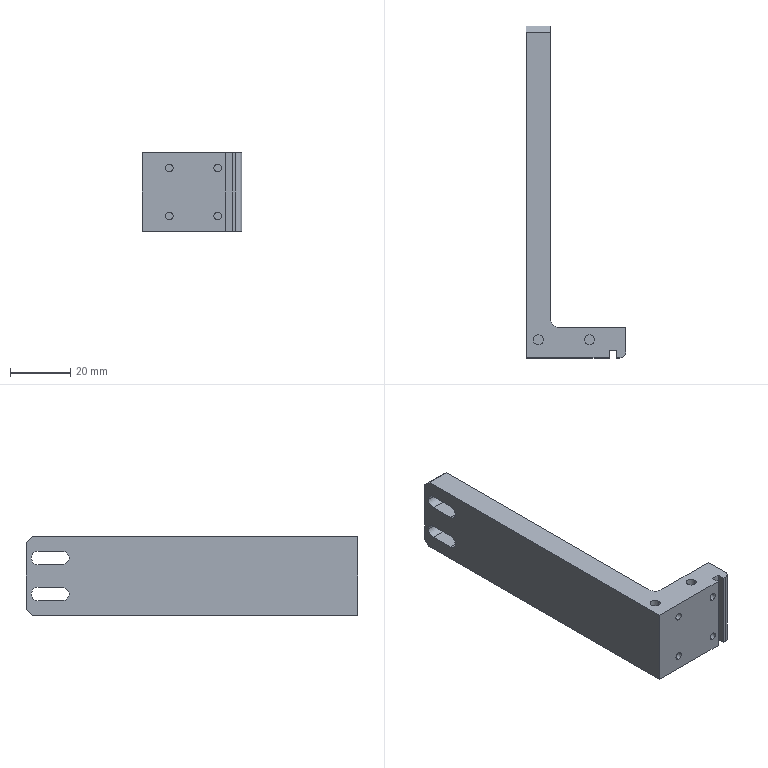Part | SolidWorks | features Fillet 2, HoleWzd 2, ICE 2, Chamfer 1, Extrusion 1, MirrorPattern 1 | 1 solid | 50 faces | box 33 x 110 x 26 mm | volume 27890 mm3 | plane 26 | cylinder 24 | commonest cylinder face diameters 2.5 x8 3.3 x8 4.5 x6 4 x1 6 x1
STEP:
#1=CARTESIAN_POINT('',(0.,108.25,-6.));
#2=VERTEX_POINT('',#1);
#3=CARTESIAN_POINT('',(0.,106.,-3.75));
#4=VERTEX_POINT('',#3);
#5=CARTESIAN_POINT('',(0.,106.,-6.));
#6=DIRECTION('',(1.,0.,0.));
#7=DIRECTION('',(0.,-1.,0.));
#8=AXIS2_PLACEMENT_3D('',#5,#6,#7);
#9=CIRCLE('',#8,2.25);
#10=EDGE_CURVE('',#2,#4,#9,.T.);
#11=ORIENTED_EDGE('',*,*,#10,.F.);
#12=CARTESIAN_POINT('',(8.,108.25,-6.));
#13=VERTEX_POINT('',#12);
#14=CARTESIAN_POINT('',(0.,108.25,-6.));
#15=DIRECTION('',(1.,0.,0.));
#16=VECTOR('',#15,1000.);
#17=LINE('',#14,#16);
#18=EDGE_CURVE('',#2,#13,#17,.T.);
#19=ORIENTED_EDGE('',*,*,#18,.T.);
#20=CARTESIAN_POINT('',(8.,106.,-3.75));
#21=VERTEX_POINT('',#20);
#22=CARTESIAN_POINT('',(8.,106.,-6.));
#23=DIRECTION('',(1.,0.,0.));
#24=DIRECTION('',(0.,-1.,0.));
#25=AXIS2_PLACEMENT_3D('',#22,#23,#24);
#26=CIRCLE('',#25,2.25);
#27=EDGE_CURVE('',#13,#21,#26,.T.);
#28=ORIENTED_EDGE('',*,*,#27,.T.);
#29=CARTESIAN_POINT('',(0.,106.,-3.75));
#30=DIRECTION('',(1.,0.,0.));
#31=VECTOR('',#30,1000.);
#32=LINE('',#29,#31);
#33=EDGE_CURVE('',#4,#21,#32,.T.);
#34=ORIENTED_EDGE('',*,*,#33,.F.);
#35=EDGE_LOOP('',(#11,#19,#28,#34));
#36=FACE_OUTER_BOUND('',#35,.T.);
#37=CARTESIAN_POINT('',(0.,106.,-6.));
#38=DIRECTION('',(1.,0.,0.));
#39=DIRECTION('',(0.,1.,0.));
#40=AXIS2_PLACEMENT_3D('',#37,#38,#39);
#41=CYLINDRICAL_SURFACE('',#40,2.25);
#42=ADVANCED_FACE('',(#36),#41,.F.);
#43=CARTESIAN_POINT('',(0.,108.25,6.));
#44=VERTEX_POINT('',#43);
#45=CARTESIAN_POINT('',(0.,106.,8.25));
#46=VERTEX_POINT('',#45);
#47=CARTESIAN_POINT('',(0.,106.,6.));
#48=DIRECTION('',(1.,0.,0.));
#49=DIRECTION('',(0.,1.,0.));
#50=AXIS2_PLACEMENT_3D('',#47,#48,#49);
#51=CIRCLE('',#50,2.25);
#52=EDGE_CURVE('',#44,#46,#51,.T.);
#53=ORIENTED_EDGE('',*,*,#52,.F.);
#54=CARTESIAN_POINT('',(8.,108.25,6.));
#55=VERTEX_POINT('',#54);
#56=CARTESIAN_POINT('',(0.,108.25,6.));
#57=DIRECTION('',(1.,0.,0.));
#58=VECTOR('',#57,1000.);
#59=LINE('',#56,#58);
#60=EDGE_CURVE('',#44,#55,#59,.T.);
#61=ORIENTED_EDGE('',*,*,#60,.T.);
#62=CARTESIAN_POINT('',(8.,106.,8.25));
#63=VERTEX_POINT('',#62);
#64=CARTESIAN_POINT('',(8.,106.,6.));
#65=DIRECTION('',(1.,0.,0.));
#66=DIRECTION('',(0.,1.,0.));
#67=AXIS2_PLACEMENT_3D('',#64,#65,#66);
#68=CIRCLE('',#67,2.25);
#69=EDGE_CURVE('',#55,#63,#68,.T.);
#70=ORIENTED_EDGE('',*,*,#69,.T.);
#71=CARTESIAN_POINT('',(0.,106.,8.25));
#72=DIRECTION('',(1.,0.,0.));
#73=VECTOR('',#72,1000.);
#74=LINE('',#71,#73);
#75=EDGE_CURVE('',#46,#63,#74,.T.);
#76=ORIENTED_EDGE('',*,*,#75,.F.);
#77=EDGE_LOOP('',(#53,#61,#70,#76));
#78=FACE_OUTER_BOUND('',#77,.T.);
#79=CARTESIAN_POINT('',(0.,106.,6.));
#80=DIRECTION('',(1.,0.,0.));
#81=DIRECTION('',(0.,1.,0.));
#82=AXIS2_PLACEMENT_3D('',#79,#80,#81);
#83=CYLINDRICAL_SURFACE('',#82,2.25);
#84=ADVANCED_FACE('',(#78),#83,.F.);
#85=CARTESIAN_POINT('',(25.,7.5,9.25));
#86=VERTEX_POINT('',#85);
#87=CARTESIAN_POINT('',(25.,7.5,6.75));
#88=VERTEX_POINT('',#87);
#89=CARTESIAN_POINT('',(25.,7.5,8.));
#90=DIRECTION('',(0.,-1.,0.));
#91=DIRECTION('',(0.,0.,-1.));
#92=AXIS2_PLACEMENT_3D('',#89,#90,#91);
#93=CIRCLE('',#92,1.25);
#94=EDGE_CURVE('',#86,#88,#93,.T.);
#95=ORIENTED_EDGE('',*,*,#94,.F.);
#96=CARTESIAN_POINT('',(25.,0.,9.25));
#97=VERTEX_POINT('',#96);
#98=CARTESIAN_POINT('',(25.,0.,9.25));
#99=DIRECTION('',(0.,-1.,0.));
#100=VECTOR('',#99,1000.);
#101=LINE('',#98,#100);
#102=EDGE_CURVE('',#86,#97,#101,.T.);
#103=ORIENTED_EDGE('',*,*,#102,.T.);
#104=CARTESIAN_POINT('',(25.,0.,6.75));
#105=VERTEX_POINT('',#104);
#106=CARTESIAN_POINT('',(25.,0.,8.));
#107=DIRECTION('',(0.,-1.,0.));
#108=DIRECTION('',(0.,0.,-1.));
#109=AXIS2_PLACEMENT_3D('',#106,#107,#108);
#110=CIRCLE('',#109,1.25);
#111=EDGE_CURVE('',#97,#105,#110,.T.);
#112=ORIENTED_EDGE('',*,*,#111,.T.);
#113=CARTESIAN_POINT('',(25.,0.,6.75));
#114=DIRECTION('',(0.,-1.,0.));
#115=VECTOR('',#114,1000.);
#116=LINE('',#113,#115);
#117=EDGE_CURVE('',#88,#105,#116,.T.);
#118=ORIENTED_EDGE('',*,*,#117,.F.);
#119=EDGE_LOOP('',(#95,#103,#112,#118));
#120=FACE_OUTER_BOUND('',#119,.T.);
#121=CARTESIAN_POINT('',(25.,0.,8.));
#122=DIRECTION('',(0.,-1.,0.));
#123=DIRECTION('',(0.,0.,-1.));
#124=AXIS2_PLACEMENT_3D('',#121,#122,#123);
#125=CYLINDRICAL_SURFACE('',#124,1.25);
#126=ADVANCED_FACE('',(#120),#125,.F.);
#127=CARTESIAN_POINT('',(9.,7.5,9.25));
#128=VERTEX_POINT('',#127);
#129=CARTESIAN_POINT('',(9.,7.5,6.75));
#130=VERTEX_POINT('',#129);
#131=CARTESIAN_POINT('',(9.,7.5,8.));
#132=DIRECTION('',(0.,-1.,0.));
#133=DIRECTION('',(0.,0.,-1.));
#134=AXIS2_PLACEMENT_3D('',#131,#132,#133);
#135=CIRCLE('',#134,1.25);
#136=EDGE_CURVE('',#128,#130,#135,.T.);
#137=ORIENTED_EDGE('',*,*,#136,.F.);
#138=CARTESIAN_POINT('',(9.,0.,9.25));
#139=VERTEX_POINT('',#138);
#140=CARTESIAN_POINT('',(9.,0.,9.25));
#141=DIRECTION('',(0.,-1.,0.));
#142=VECTOR('',#141,1000.);
#143=LINE('',#140,#142);
#144=EDGE_CURVE('',#128,#139,#143,.T.);
#145=ORIENTED_EDGE('',*,*,#144,.T.);
#146=CARTESIAN_POINT('',(9.,0.,6.75));
#147=VERTEX_POINT('',#146);
#148=CARTESIAN_POINT('',(9.,0.,8.));
#149=DIRECTION('',(0.,-1.,0.));
#150=DIRECTION('',(0.,0.,-1.));
#151=AXIS2_PLACEMENT_3D('',#148,#149,#150);
#152=CIRCLE('',#151,1.25);
#153=EDGE_CURVE('',#139,#147,#152,.T.);
#154=ORIENTED_EDGE('',*,*,#153,.T.);
#155=CARTESIAN_POINT('',(9.,0.,6.75));
#156=DIRECTION('',(0.,-1.,0.));
#157=VECTOR('',#156,1000.);
#158=LINE('',#155,#157);
#159=EDGE_CURVE('',#130,#147,#158,.T.);
#160=ORIENTED_EDGE('',*,*,#159,.F.);
#161=EDGE_LOOP('',(#137,#145,#154,#160));
#162=FACE_OUTER_BOUND('',#161,.T.);
#163=CARTESIAN_POINT('',(9.,0.,8.));
#164=DIRECTION('',(0.,-1.,0.));
#165=DIRECTION('',(0.,0.,-1.));
#166=AXIS2_PLACEMENT_3D('',#163,#164,#165);
#167=CYLINDRICAL_SURFACE('',#166,1.25);
#168=ADVANCED_FACE('',(#162),#167,.F.);
#169=CARTESIAN_POINT('',(9.,7.5,-6.75));
#170=VERTEX_POINT('',#169);
#171=CARTESIAN_POINT('',(9.,7.5,-9.25));
#172=VERTEX_POINT('',#171);
#173=CARTESIAN_POINT('',(9.,7.5,-8.));
#174=DIRECTION('',(0.,-1.,0.));
#175=DIRECTION('',(0.,0.,-1.));
#176=AXIS2_PLACEMENT_3D('',#173,#174,#175);
#177=CIRCLE('',#176,1.25);
#178=EDGE_CURVE('',#170,#172,#177,.T.);
#179=ORIENTED_EDGE('',*,*,#178,.F.);
#180=CARTESIAN_POINT('',(9.,0.,-6.75));
#181=VERTEX_POINT('',#180);
#182=CARTESIAN_POINT('',(9.,0.,-6.75));
#183=DIRECTION('',(0.,-1.,0.));
#184=VECTOR('',#183,1000.);
#185=LINE('',#182,#184);
#186=EDGE_CURVE('',#170,#181,#185,.T.);
#187=ORIENTED_EDGE('',*,*,#186,.T.);
#188=CARTESIAN_POINT('',(9.,0.,-9.25));
#189=VERTEX_POINT('',#188);
#190=CARTESIAN_POINT('',(9.,0.,-8.));
#191=DIRECTION('',(0.,-1.,0.));
#192=DIRECTION('',(0.,0.,-1.));
#193=AXIS2_PLACEMENT_3D('',#190,#191,#192);
#194=CIRCLE('',#193,1.25);
#195=EDGE_CURVE('',#181,#189,#194,.T.);
#196=ORIENTED_EDGE('',*,*,#195,.T.);
#197=CARTESIAN_POINT('',(9.,0.,-9.25));
#198=DIRECTION('',(0.,-1.,0.));
#199=VECTOR('',#198,1000.);
#200=LINE('',#197,#199);
#201=EDGE_CURVE('',#172,#189,#200,.T.);
#202=ORIENTED_EDGE('',*,*,#201,.F.);
#203=EDGE_LOOP('',(#179,#187,#196,#202));
#204=FACE_OUTER_BOUND('',#203,.T.);
#205=CARTESIAN_POINT('',(9.,0.,-8.));
#206=DIRECTION('',(0.,-1.,0.));
#207=DIRECTION('',(0.,0.,-1.));
#208=AXIS2_PLACEMENT_3D('',#205,#206,#207);
#209=CYLINDRICAL_SURFACE('',#208,1.25);
#210=ADVANCED_FACE('',(#204),#209,.F.);
#211=CARTESIAN_POINT('',(25.,7.5,-6.75));
#212=VERTEX_POINT('',#211);
#213=CARTESIAN_POINT('',(25.,7.5,-9.25));
#214=VERTEX_POINT('',#213);
#215=CARTESIAN_POINT('',(25.,7.5,-8.));
#216=DIRECTION('',(0.,-1.,0.));
#217=DIRECTION('',(0.,0.,-1.));
#218=AXIS2_PLACEMENT_3D('',#215,#216,#217);
#219=CIRCLE('',#218,1.25);
#220=EDGE_CURVE('',#212,#214,#219,.T.);
#221=ORIENTED_EDGE('',*,*,#220,.F.);
#222=CARTESIAN_POINT('',(25.,0.,-6.75));
#223=VERTEX_POINT('',#222);
#224=CARTESIAN_POINT('',(25.,0.,-6.75));
#225=DIRECTION('',(0.,-1.,0.));
#226=VECTOR('',#225,1000.);
#227=LINE('',#224,#226);
#228=EDGE_CURVE('',#212,#223,#227,.T.);
#229=ORIENTED_EDGE('',*,*,#228,.T.);
#230=CARTESIAN_POINT('',(25.,0.,-9.25));
#231=VERTEX_POINT('',#230);
#232=CARTESIAN_POINT('',(25.,0.,-8.));
#233=DIRECTION('',(0.,-1.,0.));
#234=DIRECTION('',(0.,0.,-1.));
#235=AXIS2_PLACEMENT_3D('',#232,#233,#234);
#236=CIRCLE('',#235,1.25);
#237=EDGE_CURVE('',#223,#231,#236,.T.);
#238=ORIENTED_EDGE('',*,*,#237,.T.);
#239=CARTESIAN_POINT('',(25.,0.,-9.25));
#240=DIRECTION('',(0.,-1.,0.));
#241=VECTOR('',#240,1000.);
#242=LINE('',#239,#241);
#243=EDGE_CURVE('',#214,#231,#242,.T.);
#244=ORIENTED_EDGE('',*,*,#243,.F.);
#245=EDGE_LOOP('',(#221,#229,#238,#244));
#246=FACE_OUTER_BOUND('',#245,.T.);
#247=CARTESIAN_POINT('',(25.,0.,-8.));
#248=DIRECTION('',(0.,-1.,0.));
#249=DIRECTION('',(0.,0.,-1.));
#250=AXIS2_PLACEMENT_3D('',#247,#248,#249);
#251=CYLINDRICAL_SURFACE('',#250,1.25);
#252=ADVANCED_FACE('',(#246),#251,.F.);
#253=CARTESIAN_POINT('',(22.65,6.,-2.9));
#254=VERTEX_POINT('',#253);
#255=CARTESIAN_POINT('',(19.35,6.,-2.9));
#256=VERTEX_POINT('',#255);
#257=CARTESIAN_POINT('',(21.,6.,-2.9));
#258=DIRECTION('',(0.,0.,-1.));
#259=DIRECTION('',(-1.,0.,0.));
#260=AXIS2_PLACEMENT_3D('',#257,#258,#259);
#261=CIRCLE('',#260,1.65);
#262=EDGE_CURVE('',#254,#256,#261,.T.);
#263=ORIENTED_EDGE('',*,*,#262,.F.);
#264=CARTESIAN_POINT('',(22.65,6.,-13.));
#265=VERTEX_POINT('',#264);
#266=CARTESIAN_POINT('',(22.65,6.,-13.));
#267=DIRECTION('',(0.,0.,-1.));
#268=VECTOR('',#267,1000.);
#269=LINE('',#266,#268);
#270=EDGE_CURVE('',#254,#265,#269,.T.);
#271=ORIENTED_EDGE('',*,*,#270,.T.);
#272=CARTESIAN_POINT('',(19.35,6.,-13.));
#273=VERTEX_POINT('',#272);
#274=CARTESIAN_POINT('',(21.,6.,-13.));
#275=DIRECTION('',(0.,0.,-1.));
#276=DIRECTION('',(-1.,0.,0.));
#277=AXIS2_PLACEMENT_3D('',#274,#275,#276);
#278=CIRCLE('',#277,1.65);
#279=EDGE_CURVE('',#265,#273,#278,.T.);
#280=ORIENTED_EDGE('',*,*,#279,.T.);
#281=CARTESIAN_POINT('',(19.35,6.,-13.));
#282=DIRECTION('',(0.,0.,-1.));
#283=VECTOR('',#282,1000.);
#284=LINE('',#281,#283);
#285=EDGE_CURVE('',#256,#273,#284,.T.);
#286=ORIENTED_EDGE('',*,*,#285,.F.);
#287=EDGE_LOOP('',(#263,#271,#280,#286));
#288=FACE_OUTER_BOUND('',#287,.T.);
#289=CARTESIAN_POINT('',(21.,6.,-13.));
#290=DIRECTION('',(0.,0.,-1.));
#291=DIRECTION('',(-1.,0.,0.));
#292=AXIS2_PLACEMENT_3D('',#289,#290,#291);
#293=CYLINDRICAL_SURFACE('',#292,1.65);
#294=ADVANCED_FACE('',(#288),#293,.F.);
#295=CARTESIAN_POINT('',(5.65,6.,-2.9));
#296=VERTEX_POINT('',#295);
#297=CARTESIAN_POINT('',(2.35,6.,-2.9));
#298=VERTEX_POINT('',#297);
#299=CARTESIAN_POINT('',(4.,6.,-2.9));
#300=DIRECTION('',(0.,0.,-1.));
#301=DIRECTION('',(-1.,0.,0.));
#302=AXIS2_PLACEMENT_3D('',#299,#300,#301);
#303=CIRCLE('',#302,1.65);
#304=EDGE_CURVE('',#296,#298,#303,.T.);
#305=ORIENTED_EDGE('',*,*,#304,.F.);
#306=CARTESIAN_POINT('',(5.65,6.,-13.));
#307=VERTEX_POINT('',#306);
#308=CARTESIAN_POINT('',(5.65,6.,-13.));
#309=DIRECTION('',(0.,0.,-1.));
#310=VECTOR('',#309,1000.);
#311=LINE('',#308,#310);
#312=EDGE_CURVE('',#296,#307,#311,.T.);
#313=ORIENTED_EDGE('',*,*,#312,.T.);
#314=CARTESIAN_POINT('',(2.35,6.,-13.));
#315=VERTEX_POINT('',#314);
#316=CARTESIAN_POINT('',(4.,6.,-13.));
#317=DIRECTION('',(0.,0.,-1.));
#318=DIRECTION('',(-1.,0.,0.));
#319=AXIS2_PLACEMENT_3D('',#316,#317,#318);
#320=CIRCLE('',#319,1.65);
#321=EDGE_CURVE('',#307,#315,#320,.T.);
#322=ORIENTED_EDGE('',*,*,#321,.T.);
#323=CARTESIAN_POINT('',(2.35,6.,-13.));
#324=DIRECTION('',(0.,0.,-1.));
#325=VECTOR('',#324,1000.);
#326=LINE('',#323,#325);
#327=EDGE_CURVE('',#298,#315,#326,.T.);
#328=ORIENTED_EDGE('',*,*,#327,.F.);
#329=EDGE_LOOP('',(#305,#313,#322,#328));
#330=FACE_OUTER_BOUND('',#329,.T.);
#331=CARTESIAN_POINT('',(4.,6.,-13.));
#332=DIRECTION('',(0.,0.,-1.));
#333=DIRECTION('',(-1.,0.,0.));
#334=AXIS2_PLACEMENT_3D('',#331,#332,#333);
#335=CYLINDRICAL_SURFACE('',#334,1.65);
#336=ADVANCED_FACE('',(#330),#335,.F.);
#337=CARTESIAN_POINT('',(19.35,6.,2.9));
#338=VERTEX_POINT('',#337);
#339=CARTESIAN_POINT('',(22.65,6.,2.9));
#340=VERTEX_POINT('',#339);
#341=CARTESIAN_POINT('',(21.,6.,2.9));
#342=DIRECTION('',(0.,0.,1.));
#343=DIRECTION('',(1.,0.,0.));
#344=AXIS2_PLACEMENT_3D('',#341,#342,#343);
#345=CIRCLE('',#344,1.65);
#346=EDGE_CURVE('',#338,#340,#345,.T.);
#347=ORIENTED_EDGE('',*,*,#346,.F.);
#348=CARTESIAN_POINT('',(19.35,6.,13.));
#349=VERTEX_POINT('',#348);
#350=CARTESIAN_POINT('',(19.35,6.,13.));
#351=DIRECTION('',(0.,0.,1.));
#352=VECTOR('',#351,1000.);
#353=LINE('',#350,#352);
#354=EDGE_CURVE('',#338,#349,#353,.T.);
#355=ORIENTED_EDGE('',*,*,#354,.T.);
#356=CARTESIAN_POINT('',(22.65,6.,13.));
#357=VERTEX_POINT('',#356);
#358=CARTESIAN_POINT('',(21.,6.,13.));
#359=DIRECTION('',(0.,0.,1.));
#360=DIRECTION('',(1.,0.,0.));
#361=AXIS2_PLACEMENT_3D('',#358,#359,#360);
#362=CIRCLE('',#361,1.65);
#363=EDGE_CURVE('',#349,#357,#362,.T.);
#364=ORIENTED_EDGE('',*,*,#363,.T.);
#365=CARTESIAN_POINT('',(22.65,6.,13.));
#366=DIRECTION('',(0.,0.,1.));
#367=VECTOR('',#366,1000.);
#368=LINE('',#365,#367);
#369=EDGE_CURVE('',#340,#357,#368,.T.);
#370=ORIENTED_EDGE('',*,*,#369,.F.);
#371=EDGE_LOOP('',(#347,#355,#364,#370));
#372=FACE_OUTER_BOUND('',#371,.T.);
#373=CARTESIAN_POINT('',(21.,6.,13.));
#374=DIRECTION('',(0.,0.,1.));
#375=DIRECTION('',(1.,0.,0.));
#376=AXIS2_PLACEMENT_3D('',#373,#374,#375);
#377=CYLINDRICAL_SURFACE('',#376,1.65);
#378=ADVANCED_FACE('',(#372),#377,.F.);
#379=CARTESIAN_POINT('',(2.35,6.,2.9));
#380=VERTEX_POINT('',#379);
#381=CARTESIAN_POINT('',(5.65,6.,2.9));
#382=VERTEX_POINT('',#381);
#383=CARTESIAN_POINT('',(4.,6.,2.9));
#384=DIRECTION('',(0.,0.,1.));
#385=DIRECTION('',(1.,0.,0.));
#386=AXIS2_PLACEMENT_3D('',#383,#384,#385);
#387=CIRCLE('',#386,1.65);
#388=EDGE_CURVE('',#380,#382,#387,.T.);
#389=ORIENTED_EDGE('',*,*,#388,.F.);
#390=CARTESIAN_POINT('',(2.35,6.,13.));
#391=VERTEX_POINT('',#390);
#392=CARTESIAN_POINT('',(2.35,6.,13.));
#393=DIRECTION('',(0.,0.,1.));
#394=VECTOR('',#393,1000.);
#395=LINE('',#392,#394);
#396=EDGE_CURVE('',#380,#391,#395,.T.);
#397=ORIENTED_EDGE('',*,*,#396,.T.);
#398=CARTESIAN_POINT('',(5.65,6.,13.));
#399=VERTEX_POINT('',#398);
#400=CARTESIAN_POINT('',(4.,6.,13.));
#401=DIRECTION('',(0.,0.,1.));
#402=DIRECTION('',(1.,0.,0.));
#403=AXIS2_PLACEMENT_3D('',#400,#401,#402);
#404=CIRCLE('',#403,1.65);
#405=EDGE_CURVE('',#391,#399,#404,.T.);
#406=ORIENTED_EDGE('',*,*,#405,.T.);
#407=CARTESIAN_POINT('',(5.65,6.,13.));
#408=DIRECTION('',(0.,0.,1.));
#409=VECTOR('',#408,1000.);
#410=LINE('',#407,#409);
#411=EDGE_CURVE('',#382,#399,#410,.T.);
#412=ORIENTED_EDGE('',*,*,#411,.F.);
#413=EDGE_LOOP('',(#389,#397,#406,#412));
#414=FACE_OUTER_BOUND('',#413,.T.);
#415=CARTESIAN_POINT('',(4.,6.,13.));
#416=DIRECTION('',(0.,0.,1.));
#417=DIRECTION('',(1.,0.,0.));
#418=AXIS2_PLACEMENT_3D('',#415,#416,#417);
#419=CYLINDRICAL_SURFACE('',#418,1.65);
#420=ADVANCED_FACE('',(#414),#419,.F.);
#421=CARTESIAN_POINT('',(30.,0.,-13.));
#422=VERTEX_POINT('',#421);
#423=CARTESIAN_POINT('',(31.,0.,-13.));
#424=VERTEX_POINT('',#423);
#425=CARTESIAN_POINT('',(0.,0.,-13.));
#426=DIRECTION('',(1.,0.,0.));
#427=VECTOR('',#426,1000.);
#428=LINE('',#425,#427);
#429=EDGE_CURVE('',#422,#424,#428,.T.);
#430=ORIENTED_EDGE('',*,*,#429,.T.);
#431=CARTESIAN_POINT('',(31.,0.,13.));
#432=VERTEX_POINT('',#431);
#433=CARTESIAN_POINT('',(31.,0.,13.));
#434=DIRECTION('',(0.,0.,1.));
#435=VECTOR('',#434,1000.);
#436=LINE('',#433,#435);
#437=EDGE_CURVE('',#424,#432,#436,.T.);
#438=ORIENTED_EDGE('',*,*,#437,.T.);
#439=CARTESIAN_POINT('',(30.,0.,13.));
#440=VERTEX_POINT('',#439);
#441=CARTESIAN_POINT('',(0.,0.,13.));
#442=DIRECTION('',(1.,0.,0.));
#443=VECTOR('',#442,1000.);
#444=LINE('',#441,#443);
#445=EDGE_CURVE('',#440,#432,#444,.T.);
#446=ORIENTED_EDGE('',*,*,#445,.F.);
#447=CARTESIAN_POINT('',(30.,0.,-13.));
#448=DIRECTION('',(0.,0.,1.));
#449=VECTOR('',#448,1000.);
#450=LINE('',#447,#449);
#451=EDGE_CURVE('',#422,#440,#450,.T.);
#452=ORIENTED_EDGE('',*,*,#451,.F.);
#453=EDGE_LOOP('',(#430,#438,#446,#452));
#454=FACE_OUTER_BOUND('',#453,.T.);
#455=CARTESIAN_POINT('',(0.,0.,13.));
#456=DIRECTION('',(0.,1.,0.));
#457=DIRECTION('',(0.,0.,1.));
#458=AXIS2_PLACEMENT_3D('',#455,#456,#457);
#459=PLANE('',#458);
#460=ADVANCED_FACE('',(#454),#459,.F.);
#461=CARTESIAN_POINT('',(0.,98.,-8.25));
#462=VERTEX_POINT('',#461);
#463=CARTESIAN_POINT('',(0.,106.,-8.25));
#464=VERTEX_POINT('',#463);
#465=CARTESIAN_POINT('',(0.,106.,-8.25));
#466=DIRECTION('',(0.,1.,0.));
#467=VECTOR('',#466,1000.);
#468=LINE('',#465,#467);
#469=EDGE_CURVE('',#462,#464,#468,.T.);
#470=ORIENTED_EDGE('',*,*,#469,.T.);
#471=CARTESIAN_POINT('',(0.,106.,-6.));
#472=DIRECTION('',(1.,0.,0.));
#473=DIRECTION('',(0.,-1.,0.));
#474=AXIS2_PLACEMENT_3D('',#471,#472,#473);
#475=CIRCLE('',#474,2.25);
#476=EDGE_CURVE('',#464,#2,#475,.T.);
#477=ORIENTED_EDGE('',*,*,#476,.T.);
#478=ORIENTED_EDGE('',*,*,#10,.T.);
#479=CARTESIAN_POINT('',(0.,98.,-3.75));
#480=VERTEX_POINT('',#479);
#481=CARTESIAN_POINT('',(0.,106.,-3.75));
#482=DIRECTION('',(0.,-1.,0.));
#483=VECTOR('',#482,1000.);
#484=LINE('',#481,#483);
#485=EDGE_CURVE('',#4,#480,#484,.T.);
#486=ORIENTED_EDGE('',*,*,#485,.T.);
#487=CARTESIAN_POINT('',(0.,98.,-6.));
#488=DIRECTION('',(1.,0.,0.));
#489=DIRECTION('',(0.,-1.,0.));
#490=AXIS2_PLACEMENT_3D('',#487,#488,#489);
#491=CIRCLE('',#490,2.25);
#492=EDGE_CURVE('',#480,#462,#491,.T.);
#493=ORIENTED_EDGE('',*,*,#492,.T.);
#494=EDGE_LOOP('',(#470,#477,#478,#486,#493));
#495=FACE_BOUND('',#494,.T.);
#496=CARTESIAN_POINT('',(0.,98.,3.75));
#497=VERTEX_POINT('',#496);
#498=CARTESIAN_POINT('',(0.,106.,3.75));
#499=VERTEX_POINT('',#498);
#500=CARTESIAN_POINT('',(0.,106.,3.75));
#501=DIRECTION('',(0.,1.,0.));
#502=VECTOR('',#501,1000.);
#503=LINE('',#500,#502);
#504=EDGE_CURVE('',#497,#499,#503,.T.);
#505=ORIENTED_EDGE('',*,*,#504,.T.);
#506=CARTESIAN_POINT('',(0.,106.,6.));
#507=DIRECTION('',(1.,0.,0.));
#508=DIRECTION('',(0.,1.,0.));
#509=AXIS2_PLACEMENT_3D('',#506,#507,#508);
#510=CIRCLE('',#509,2.25);
#511=EDGE_CURVE('',#499,#44,#510,.T.);
#512=ORIENTED_EDGE('',*,*,#511,.T.);
#513=ORIENTED_EDGE('',*,*,#52,.T.);
#514=CARTESIAN_POINT('',(0.,98.,8.25));
#515=VERTEX_POINT('',#514);
#516=CARTESIAN_POINT('',(0.,106.,8.25));
#517=DIRECTION('',(0.,-1.,0.));
#518=VECTOR('',#517,1000.);
#519=LINE('',#516,#518);
#520=EDGE_CURVE('',#46,#515,#519,.T.);
#521=ORIENTED_EDGE('',*,*,#520,.T.);
#522=CARTESIAN_POINT('',(0.,98.,6.));
#523=DIRECTION('',(1.,0.,0.));
#524=DIRECTION('',(0.,1.,0.));
#525=AXIS2_PLACEMENT_3D('',#522,#523,#524);
#526=CIRCLE('',#525,2.25);
#527=EDGE_CURVE('',#515,#497,#526,.T.);
#528=ORIENTED_EDGE('',*,*,#527,.T.);
#529=EDGE_LOOP('',(#505,#512,#513,#521,#528));
#530=FACE_BOUND('',#529,.T.);
#531=CARTESIAN_POINT('',(0.,108.,13.));
#532=VERTEX_POINT('',#531);
#533=CARTESIAN_POINT('',(0.,0.,13.));
#534=VERTEX_POINT('',#533);
#535=CARTESIAN_POINT('',(0.,0.,13.));
#536=DIRECTION('',(0.,-1.,0.));
#537=VECTOR('',#536,1000.);
#538=LINE('',#535,#537);
#539=EDGE_CURVE('',#532,#534,#538,.T.);
#540=ORIENTED_EDGE('',*,*,#539,.F.);
#541=CARTESIAN_POINT('',(0.,110.,11.));
#542=VERTEX_POINT('',#541);
#543=CARTESIAN_POINT('',(0.,108.,13.));
#544=DIRECTION('',(0.,0.7071,-0.7071));
#545=VECTOR('',#544,1000.);
#546=LINE('',#543,#545);
#547=EDGE_CURVE('',#532,#542,#546,.T.);
#548=ORIENTED_EDGE('',*,*,#547,.T.);
#549=CARTESIAN_POINT('',(0.,110.,-11.));
#550=VERTEX_POINT('',#549);
#551=CARTESIAN_POINT('',(0.,110.,13.));
#552=DIRECTION('',(0.,0.,-1.));
#553=VECTOR('',#552,1000.);
#554=LINE('',#551,#553);
#555=EDGE_CURVE('',#542,#550,#554,.T.);
#556=ORIENTED_EDGE('',*,*,#555,.T.);
#557=CARTESIAN_POINT('',(0.,108.,-13.));
#558=VERTEX_POINT('',#557);
#559=CARTESIAN_POINT('',(0.,110.,-11.));
#560=DIRECTION('',(0.,-0.7071,-0.7071));
#561=VECTOR('',#560,1000.);
#562=LINE('',#559,#561);
#563=EDGE_CURVE('',#550,#558,#562,.T.);
#564=ORIENTED_EDGE('',*,*,#563,.T.);
#565=CARTESIAN_POINT('',(0.,0.,-13.));
#566=VERTEX_POINT('',#565);
#567=CARTESIAN_POINT('',(0.,0.,-13.));
#568=DIRECTION('',(0.,-1.,0.));
#569=VECTOR('',#568,1000.);
#570=LINE('',#567,#569);
#571=EDGE_CURVE('',#558,#566,#570,.T.);
#572=ORIENTED_EDGE('',*,*,#571,.T.);
#573=CARTESIAN_POINT('',(0.,0.,13.));
#574=DIRECTION('',(0.,0.,-1.));
#575=VECTOR('',#574,1000.);
#576=LINE('',#573,#575);
#577=EDGE_CURVE('',#534,#566,#576,.T.);
#578=ORIENTED_EDGE('',*,*,#577,.F.);
#579=EDGE_LOOP('',(#540,#548,#556,#564,#572,#578));
#580=FACE_OUTER_BOUND('',#579,.T.);
#581=CARTESIAN_POINT('',(0.,0.,13.));
#582=DIRECTION('',(1.,0.,0.));
#583=DIRECTION('',(0.,0.,-1.));
#584=AXIS2_PLACEMENT_3D('',#581,#582,#583);
#585=PLANE('',#584);
#586=ADVANCED_FACE('',(#495,#530,#580),#585,.F.);
#587=CARTESIAN_POINT('',(25.,0.,8.));
#588=DIRECTION('',(0.,-1.,0.));
#589=DIRECTION('',(0.,0.,-1.));
#590=AXIS2_PLACEMENT_3D('',#587,#588,#589);
#591=CIRCLE('',#590,1.25);
#592=EDGE_CURVE('',#105,#97,#591,.T.);
#593=ORIENTED_EDGE('',*,*,#592,.F.);
#594=ORIENTED_EDGE('',*,*,#111,.F.);
#595=EDGE_LOOP('',(#593,#594));
#596=FACE_BOUND('',#595,.T.);
#597=CARTESIAN_POINT('',(9.,0.,8.));
#598=DIRECTION('',(0.,-1.,0.));
#599=DIRECTION('',(0.,0.,-1.));
#600=AXIS2_PLACEMENT_3D('',#597,#598,#599);
#601=CIRCLE('',#600,1.25);
#602=EDGE_CURVE('',#147,#139,#601,.T.);
#603=ORIENTED_EDGE('',*,*,#602,.F.);
#604=ORIENTED_EDGE('',*,*,#153,.F.);
#605=EDGE_LOOP('',(#603,#604));
#606=FACE_BOUND('',#605,.T.);
#607=CARTESIAN_POINT('',(9.,0.,-8.));
#608=DIRECTION('',(0.,-1.,0.));
#609=DIRECTION('',(0.,0.,-1.));
#610=AXIS2_PLACEMENT_3D('',#607,#608,#609);
#611=CIRCLE('',#610,1.25);
#612=EDGE_CURVE('',#189,#181,#611,.T.);
#613=ORIENTED_EDGE('',*,*,#612,.F.);
#614=ORIENTED_EDGE('',*,*,#195,.F.);
#615=EDGE_LOOP('',(#613,#614));
#616=FACE_BOUND('',#615,.T.);
#617=CARTESIAN_POINT('',(25.,0.,-8.));
#618=DIRECTION('',(0.,-1.,0.));
#619=DIRECTION('',(0.,0.,-1.));
#620=AXIS2_PLACEMENT_3D('',#617,#618,#619);
#621=CIRCLE('',#620,1.25);
#622=EDGE_CURVE('',#231,#223,#621,.T.);
#623=ORIENTED_EDGE('',*,*,#622,.F.);
#624=ORIENTED_EDGE('',*,*,#237,.F.);
#625=EDGE_LOOP('',(#623,#624));
#626=FACE_BOUND('',#625,.T.);
#627=CARTESIAN_POINT('',(27.5,0.,-13.));
#628=VERTEX_POINT('',#627);
#629=CARTESIAN_POINT('',(0.,0.,-13.));
#630=DIRECTION('',(1.,0.,0.));
#631=VECTOR('',#630,1000.);
#632=LINE('',#629,#631);
#633=EDGE_CURVE('',#566,#628,#632,.T.);
#634=ORIENTED_EDGE('',*,*,#633,.T.);
#635=CARTESIAN_POINT('',(27.5,0.,13.));
#636=VERTEX_POINT('',#635);
#637=CARTESIAN_POINT('',(27.5,0.,-13.));
#638=DIRECTION('',(0.,0.,1.));
#639=VECTOR('',#638,1000.);
#640=LINE('',#637,#639);
#641=EDGE_CURVE('',#628,#636,#640,.T.);
#642=ORIENTED_EDGE('',*,*,#641,.T.);
#643=CARTESIAN_POINT('',(0.,0.,13.));
#644=DIRECTION('',(1.,0.,0.));
#645=VECTOR('',#644,1000.);
#646=LINE('',#643,#645);
#647=EDGE_CURVE('',#534,#636,#646,.T.);
#648=ORIENTED_EDGE('',*,*,#647,.F.);
#649=ORIENTED_EDGE('',*,*,#577,.T.);
#650=EDGE_LOOP('',(#634,#642,#648,#649));
#651=FACE_OUTER_BOUND('',#650,.T.);
#652=CARTESIAN_POINT('',(0.,0.,13.));
#653=DIRECTION('',(0.,1.,0.));
#654=DIRECTION('',(0.,0.,1.));
#655=AXIS2_PLACEMENT_3D('',#652,#653,#654);
#656=PLANE('',#655);
#657=ADVANCED_FACE('',(#596,#606,#616,#626,#651),#656,.F.);
#658=CARTESIAN_POINT('',(33.,2.,13.));
#659=VERTEX_POINT('',#658);
#660=CARTESIAN_POINT('',(33.,10.,13.));
#661=VERTEX_POINT('',#660);
#662=CARTESIAN_POINT('',(33.,0.,13.));
#663=DIRECTION('',(0.,1.,0.));
#664=VECTOR('',#663,1000.);
#665=LINE('',#662,#664);
#666=EDGE_CURVE('',#659,#661,#665,.T.);
#667=ORIENTED_EDGE('',*,*,#666,.F.);
#668=CARTESIAN_POINT('',(33.,2.,-13.));
#669=VERTEX_POINT('',#668);
#670=CARTESIAN_POINT('',(33.,2.,13.));
#671=DIRECTION('',(0.,0.,-1.));
#672=VECTOR('',#671,1000.);
#673=LINE('',#670,#672);
#674=EDGE_CURVE('',#659,#669,#673,.T.);
#675=ORIENTED_EDGE('',*,*,#674,.T.);
#676=CARTESIAN_POINT('',(33.,10.,-13.));
#677=VERTEX_POINT('',#676);
#678=CARTESIAN_POINT('',(33.,0.,-13.));
#679=DIRECTION('',(0.,1.,0.));
#680=VECTOR('',#679,1000.);
#681=LINE('',#678,#680);
#682=EDGE_CURVE('',#669,#677,#681,.T.);
#683=ORIENTED_EDGE('',*,*,#682,.T.);
#684=CARTESIAN_POINT('',(33.,10.,13.));
#685=DIRECTION('',(0.,0.,-1.));
#686=VECTOR('',#685,1000.);
#687=LINE('',#684,#686);
#688=EDGE_CURVE('',#661,#677,#687,.T.);
#689=ORIENTED_EDGE('',*,*,#688,.F.);
#690=EDGE_LOOP('',(#667,#675,#683,#689));
#691=FACE_OUTER_BOUND('',#690,.T.);
#692=CARTESIAN_POINT('',(33.,0.,13.));
#693=DIRECTION('',(-1.,0.,0.));
#694=DIRECTION('',(0.,0.,1.));
#695=AXIS2_PLACEMENT_3D('',#692,#693,#694);
#696=PLANE('',#695);
#697=ADVANCED_FACE('',(#691),#696,.F.);
#698=CARTESIAN_POINT('',(11.,10.,-13.));
#699=VERTEX_POINT('',#698);
#700=CARTESIAN_POINT('',(33.,10.,-13.));
#701=DIRECTION('',(-1.,0.,0.));
#702=VECTOR('',#701,1000.);
#703=LINE('',#700,#702);
#704=EDGE_CURVE('',#677,#699,#703,.T.);
#705=ORIENTED_EDGE('',*,*,#704,.T.);
#706=CARTESIAN_POINT('',(11.,10.,13.));
#707=VERTEX_POINT('',#706);
#708=CARTESIAN_POINT('',(11.,10.,13.));
#709=DIRECTION('',(0.,0.,1.));
#710=VECTOR('',#709,1000.);
#711=LINE('',#708,#710);
#712=EDGE_CURVE('',#699,#707,#711,.T.);
#713=ORIENTED_EDGE('',*,*,#712,.T.);
#714=CARTESIAN_POINT('',(33.,10.,13.));
#715=DIRECTION('',(-1.,0.,0.));
#716=VECTOR('',#715,1000.);
#717=LINE('',#714,#716);
#718=EDGE_CURVE('',#661,#707,#717,.T.);
#719=ORIENTED_EDGE('',*,*,#718,.F.);
#720=ORIENTED_EDGE('',*,*,#688,.T.);
#721=EDGE_LOOP('',(#705,#713,#719,#720));
#722=FACE_OUTER_BOUND('',#721,.T.);
#723=CARTESIAN_POINT('',(33.,10.,13.));
#724=DIRECTION('',(0.,-1.,0.));
#725=DIRECTION('',(1.,0.,0.));
#726=AXIS2_PLACEMENT_3D('',#723,#724,#725);
#727=PLANE('',#726);
#728=ADVANCED_FACE('',(#722),#727,.F.);
#729=CARTESIAN_POINT('',(8.,98.,-3.75));
#730=VERTEX_POINT('',#729);
#731=CARTESIAN_POINT('',(8.,106.,-3.75));
#732=DIRECTION('',(0.,-1.,0.));
#733=VECTOR('',#732,1000.);
#734=LINE('',#731,#733);
#735=EDGE_CURVE('',#21,#730,#734,.T.);
#736=ORIENTED_EDGE('',*,*,#735,.F.);
#737=ORIENTED_EDGE('',*,*,#27,.F.);
#738=CARTESIAN_POINT('',(8.,106.,-8.25));
#739=VERTEX_POINT('',#738);
#740=CARTESIAN_POINT('',(8.,106.,-6.));
#741=DIRECTION('',(1.,0.,0.));
#742=DIRECTION('',(0.,-1.,0.));
#743=AXIS2_PLACEMENT_3D('',#740,#741,#742);
#744=CIRCLE('',#743,2.25);
#745=EDGE_CURVE('',#739,#13,#744,.T.);
#746=ORIENTED_EDGE('',*,*,#745,.F.);
#747=CARTESIAN_POINT('',(8.,98.,-8.25));
#748=VERTEX_POINT('',#747);
#749=CARTESIAN_POINT('',(8.,106.,-8.25));
#750=DIRECTION('',(0.,1.,0.));
#751=VECTOR('',#750,1000.);
#752=LINE('',#749,#751);
#753=EDGE_CURVE('',#748,#739,#752,.T.);
#754=ORIENTED_EDGE('',*,*,#753,.F.);
#755=CARTESIAN_POINT('',(8.,98.,-6.));
#756=DIRECTION('',(1.,0.,0.));
#757=DIRECTION('',(0.,-1.,0.));
#758=AXIS2_PLACEMENT_3D('',#755,#756,#757);
#759=CIRCLE('',#758,2.25);
#760=EDGE_CURVE('',#730,#748,#759,.T.);
#761=ORIENTED_EDGE('',*,*,#760,.F.);
#762=EDGE_LOOP('',(#736,#737,#746,#754,#761));
#763=FACE_BOUND('',#762,.T.);
#764=CARTESIAN_POINT('',(8.,98.,8.25));
#765=VERTEX_POINT('',#764);
#766=CARTESIAN_POINT('',(8.,106.,8.25));
#767=DIRECTION('',(0.,-1.,0.));
#768=VECTOR('',#767,1000.);
#769=LINE('',#766,#768);
#770=EDGE_CURVE('',#63,#765,#769,.T.);
#771=ORIENTED_EDGE('',*,*,#770,.F.);
#772=ORIENTED_EDGE('',*,*,#69,.F.);
#773=CARTESIAN_POINT('',(8.,106.,3.75));
#774=VERTEX_POINT('',#773);
#775=CARTESIAN_POINT('',(8.,106.,6.));
#776=DIRECTION('',(1.,0.,0.));
#777=DIRECTION('',(0.,1.,0.));
#778=AXIS2_PLACEMENT_3D('',#775,#776,#777);
#779=CIRCLE('',#778,2.25);
#780=EDGE_CURVE('',#774,#55,#779,.T.);
#781=ORIENTED_EDGE('',*,*,#780,.F.);
#782=CARTESIAN_POINT('',(8.,98.,3.75));
#783=VERTEX_POINT('',#782);
#784=CARTESIAN_POINT('',(8.,106.,3.75));
#785=DIRECTION('',(0.,1.,0.));
#786=VECTOR('',#785,1000.);
#787=LINE('',#784,#786);
#788=EDGE_CURVE('',#783,#774,#787,.T.);
#789=ORIENTED_EDGE('',*,*,#788,.F.);
#790=CARTESIAN_POINT('',(8.,98.,6.));
#791=DIRECTION('',(1.,0.,0.));
#792=DIRECTION('',(0.,1.,0.));
#793=AXIS2_PLACEMENT_3D('',#790,#791,#792);
#794=CIRCLE('',#793,2.25);
#795=EDGE_CURVE('',#765,#783,#794,.T.);
#796=ORIENTED_EDGE('',*,*,#795,.F.);
#797=EDGE_LOOP('',(#771,#772,#781,#789,#796));
#798=FACE_BOUND('',#797,.T.);
#799=CARTESIAN_POINT('',(8.,110.,11.));
#800=VERTEX_POINT('',#799);
#801=CARTESIAN_POINT('',(8.,110.,-11.));
#802=VERTEX_POINT('',#801);
#803=CARTESIAN_POINT('',(8.,110.,13.));
#804=DIRECTION('',(0.,0.,-1.));
#805=VECTOR('',#804,1000.);
#806=LINE('',#803,#805);
#807=EDGE_CURVE('',#800,#802,#806,.T.);
#808=ORIENTED_EDGE('',*,*,#807,.F.);
#809=CARTESIAN_POINT('',(8.,108.,13.));
#810=VERTEX_POINT('',#809);
#811=CARTESIAN_POINT('',(8.,108.,13.));
#812=DIRECTION('',(0.,-0.7071,0.7071));
#813=VECTOR('',#812,1000.);
#814=LINE('',#811,#813);
#815=EDGE_CURVE('',#800,#810,#814,.T.);
#816=ORIENTED_EDGE('',*,*,#815,.T.);
#817=CARTESIAN_POINT('',(8.,13.,13.));
#818=VERTEX_POINT('',#817);
#819=CARTESIAN_POINT('',(8.,110.,13.));
#820=DIRECTION('',(0.,1.,0.));
#821=VECTOR('',#820,1000.);
#822=LINE('',#819,#821);
#823=EDGE_CURVE('',#818,#810,#822,.T.);
#824=ORIENTED_EDGE('',*,*,#823,.F.);
#825=CARTESIAN_POINT('',(8.,13.,-13.));
#826=VERTEX_POINT('',#825);
#827=CARTESIAN_POINT('',(8.,13.,-13.));
#828=DIRECTION('',(0.,0.,-1.));
#829=VECTOR('',#828,1000.);
#830=LINE('',#827,#829);
#831=EDGE_CURVE('',#818,#826,#830,.T.);
#832=ORIENTED_EDGE('',*,*,#831,.T.);
#833=CARTESIAN_POINT('',(8.,108.,-13.));
#834=VERTEX_POINT('',#833);
#835=CARTESIAN_POINT('',(8.,110.,-13.));
#836=DIRECTION('',(0.,1.,0.));
#837=VECTOR('',#836,1000.);
#838=LINE('',#835,#837);
#839=EDGE_CURVE('',#826,#834,#838,.T.);
#840=ORIENTED_EDGE('',*,*,#839,.T.);
#841=CARTESIAN_POINT('',(8.,110.,-11.));
#842=DIRECTION('',(0.,0.7071,0.7071));
#843=VECTOR('',#842,1000.);
#844=LINE('',#841,#843);
#845=EDGE_CURVE('',#834,#802,#844,.T.);
#846=ORIENTED_EDGE('',*,*,#845,.T.);
#847=EDGE_LOOP('',(#808,#816,#824,#832,#840,#846));
#848=FACE_OUTER_BOUND('',#847,.T.);
#849=CARTESIAN_POINT('',(8.,110.,13.));
#850=DIRECTION('',(-1.,0.,0.));
#851=DIRECTION('',(0.,-1.,0.));
#852=AXIS2_PLACEMENT_3D('',#849,#850,#851);
#853=PLANE('',#852);
#854=ADVANCED_FACE('',(#763,#798,#848),#853,.F.);
#855=ORIENTED_EDGE('',*,*,#555,.F.);
#856=CARTESIAN_POINT('',(0.,110.,11.));
#857=DIRECTION('',(1.,0.,0.));
#858=VECTOR('',#857,1000.);
#859=LINE('',#856,#858);
#860=EDGE_CURVE('',#542,#800,#859,.T.);
#861=ORIENTED_EDGE('',*,*,#860,.T.);
#862=ORIENTED_EDGE('',*,*,#807,.T.);
#863=CARTESIAN_POINT('',(0.,110.,-11.));
#864=DIRECTION('',(-1.,0.,0.));
#865=VECTOR('',#864,1000.);
#866=LINE('',#863,#865);
#867=EDGE_CURVE('',#802,#550,#866,.T.);
#868=ORIENTED_EDGE('',*,*,#867,.T.);
#869=EDGE_LOOP('',(#855,#861,#862,#868));
#870=FACE_OUTER_BOUND('',#869,.T.);
#871=CARTESIAN_POINT('',(0.,110.,13.));
#872=DIRECTION('',(0.,-1.,0.));
#873=DIRECTION('',(0.,0.,-1.));
#874=AXIS2_PLACEMENT_3D('',#871,#872,#873);
#875=PLANE('',#874);
#876=ADVANCED_FACE('',(#870),#875,.F.);
#877=CARTESIAN_POINT('',(21.,6.,13.));
#878=DIRECTION('',(0.,0.,1.));
#879=DIRECTION('',(1.,0.,0.));
#880=AXIS2_PLACEMENT_3D('',#877,#878,#879);
#881=CIRCLE('',#880,1.65);
#882=EDGE_CURVE('',#357,#349,#881,.T.);
#883=ORIENTED_EDGE('',*,*,#882,.F.);
#884=ORIENTED_EDGE('',*,*,#363,.F.);
#885=EDGE_LOOP('',(#883,#884));
#886=FACE_BOUND('',#885,.T.);
#887=CARTESIAN_POINT('',(4.,6.,13.));
#888=DIRECTION('',(0.,0.,1.));
#889=DIRECTION('',(1.,0.,0.));
#890=AXIS2_PLACEMENT_3D('',#887,#888,#889);
#891=CIRCLE('',#890,1.65);
#892=EDGE_CURVE('',#399,#391,#891,.T.);
#893=ORIENTED_EDGE('',*,*,#892,.F.);
#894=ORIENTED_EDGE('',*,*,#405,.F.);
#895=EDGE_LOOP('',(#893,#894));
#896=FACE_BOUND('',#895,.T.);
#897=ORIENTED_EDGE('',*,*,#823,.T.);
#898=CARTESIAN_POINT('',(0.,108.,13.));
#899=DIRECTION('',(-1.,0.,0.));
#900=VECTOR('',#899,1000.);
#901=LINE('',#898,#900);
#902=EDGE_CURVE('',#810,#532,#901,.T.);
#903=ORIENTED_EDGE('',*,*,#902,.T.);
#904=ORIENTED_EDGE('',*,*,#539,.T.);
#905=ORIENTED_EDGE('',*,*,#647,.T.);
#906=CARTESIAN_POINT('',(27.5,2.5,13.));
#907=VERTEX_POINT('',#906);
#908=CARTESIAN_POINT('',(27.5,0.,13.));
#909=DIRECTION('',(0.,-1.,0.));
#910=VECTOR('',#909,1000.);
#911=LINE('',#908,#910);
#912=EDGE_CURVE('',#907,#636,#911,.T.);
#913=ORIENTED_EDGE('',*,*,#912,.F.);
#914=CARTESIAN_POINT('',(30.,2.5,13.));
#915=VERTEX_POINT('',#914);
#916=CARTESIAN_POINT('',(30.,2.5,13.));
#917=DIRECTION('',(-1.,0.,0.));
#918=VECTOR('',#917,1000.);
#919=LINE('',#916,#918);
#920=EDGE_CURVE('',#915,#907,#919,.T.);
#921=ORIENTED_EDGE('',*,*,#920,.F.);
#922=CARTESIAN_POINT('',(30.,0.,13.));
#923=DIRECTION('',(0.,1.,0.));
#924=VECTOR('',#923,1000.);
#925=LINE('',#922,#924);
#926=EDGE_CURVE('',#440,#915,#925,.T.);
#927=ORIENTED_EDGE('',*,*,#926,.F.);
#928=ORIENTED_EDGE('',*,*,#445,.T.);
#929=CARTESIAN_POINT('',(31.,2.,13.));
#930=DIRECTION('',(0.,0.,1.));
#931=DIRECTION('',(-1.,0.,0.));
#932=AXIS2_PLACEMENT_3D('',#929,#930,#931);
#933=CIRCLE('',#932,2.);
#934=EDGE_CURVE('',#432,#659,#933,.T.);
#935=ORIENTED_EDGE('',*,*,#934,.T.);
#936=ORIENTED_EDGE('',*,*,#666,.T.);
#937=ORIENTED_EDGE('',*,*,#718,.T.);
#938=CARTESIAN_POINT('',(11.,13.,13.));
#939=DIRECTION('',(0.,0.,-1.));
#940=DIRECTION('',(-1.,0.,0.));
#941=AXIS2_PLACEMENT_3D('',#938,#939,#940);
#942=CIRCLE('',#941,3.);
#943=EDGE_CURVE('',#707,#818,#942,.T.);
#944=ORIENTED_EDGE('',*,*,#943,.T.);
#945=EDGE_LOOP('',(#897,#903,#904,#905,#913,#921,#927,#928,#935,#936,#937,#944));
#946=FACE_OUTER_BOUND('',#945,.T.);
#947=CARTESIAN_POINT('',(0.,110.,13.));
#948=DIRECTION('',(0.,0.,-1.));
#949=DIRECTION('',(-1.,0.,0.));
#950=AXIS2_PLACEMENT_3D('',#947,#948,#949);
#951=PLANE('',#950);
#952=ADVANCED_FACE('',(#886,#896,#946),#951,.F.);
#953=CARTESIAN_POINT('',(21.,6.,-13.));
#954=DIRECTION('',(0.,0.,-1.));
#955=DIRECTION('',(-1.,0.,0.));
#956=AXIS2_PLACEMENT_3D('',#953,#954,#955);
#957=CIRCLE('',#956,1.65);
#958=EDGE_CURVE('',#273,#265,#957,.T.);
#959=ORIENTED_EDGE('',*,*,#958,.F.);
#960=ORIENTED_EDGE('',*,*,#279,.F.);
#961=EDGE_LOOP('',(#959,#960));
#962=FACE_BOUND('',#961,.T.);
#963=CARTESIAN_POINT('',(4.,6.,-13.));
#964=DIRECTION('',(0.,0.,-1.));
#965=DIRECTION('',(-1.,0.,0.));
#966=AXIS2_PLACEMENT_3D('',#963,#964,#965);
#967=CIRCLE('',#966,1.65);
#968=EDGE_CURVE('',#315,#307,#967,.T.);
#969=ORIENTED_EDGE('',*,*,#968,.F.);
#970=ORIENTED_EDGE('',*,*,#321,.F.);
#971=EDGE_LOOP('',(#969,#970));
#972=FACE_BOUND('',#971,.T.);
#973=ORIENTED_EDGE('',*,*,#571,.F.);
#974=CARTESIAN_POINT('',(8.,108.,-13.));
#975=DIRECTION('',(1.,0.,0.));
#976=VECTOR('',#975,1000.);
#977=LINE('',#974,#976);
#978=EDGE_CURVE('',#558,#834,#977,.T.);
#979=ORIENTED_EDGE('',*,*,#978,.T.);
#980=ORIENTED_EDGE('',*,*,#839,.F.);
#981=CARTESIAN_POINT('',(11.,13.,-13.));
#982=DIRECTION('',(0.,0.,1.));
#983=DIRECTION('',(-1.,0.,0.));
#984=AXIS2_PLACEMENT_3D('',#981,#982,#983);
#985=CIRCLE('',#984,3.);
#986=EDGE_CURVE('',#826,#699,#985,.T.);
#987=ORIENTED_EDGE('',*,*,#986,.T.);
#988=ORIENTED_EDGE('',*,*,#704,.F.);
#989=ORIENTED_EDGE('',*,*,#682,.F.);
#990=CARTESIAN_POINT('',(31.,2.,-13.));
#991=DIRECTION('',(0.,0.,-1.));
#992=DIRECTION('',(-1.,0.,0.));
#993=AXIS2_PLACEMENT_3D('',#990,#991,#992);
#994=CIRCLE('',#993,2.);
#995=EDGE_CURVE('',#669,#424,#994,.T.);
#996=ORIENTED_EDGE('',*,*,#995,.T.);
#997=ORIENTED_EDGE('',*,*,#429,.F.);
#998=CARTESIAN_POINT('',(30.,2.5,-13.));
#999=VERTEX_POINT('',#998);
#1000=CARTESIAN_POINT('',(30.,0.,-13.));
#1001=DIRECTION('',(0.,1.,0.));
#1002=VECTOR('',#1001,1000.);
#1003=LINE('',#1000,#1002);
#1004=EDGE_CURVE('',#422,#999,#1003,.T.);
#1005=ORIENTED_EDGE('',*,*,#1004,.T.);
#1006=CARTESIAN_POINT('',(27.5,2.5,-13.));
#1007=VERTEX_POINT('',#1006);
#1008=CARTESIAN_POINT('',(30.,2.5,-13.));
#1009=DIRECTION('',(-1.,0.,0.));
#1010=VECTOR('',#1009,1000.);
#1011=LINE('',#1008,#1010);
#1012=EDGE_CURVE('',#999,#1007,#1011,.T.);
#1013=ORIENTED_EDGE('',*,*,#1012,.T.);
#1014=CARTESIAN_POINT('',(27.5,0.,-13.));
#1015=DIRECTION('',(0.,-1.,0.));
#1016=VECTOR('',#1015,1000.);
#1017=LINE('',#1014,#1016);
#1018=EDGE_CURVE('',#1007,#628,#1017,.T.);
#1019=ORIENTED_EDGE('',*,*,#1018,.T.);
#1020=ORIENTED_EDGE('',*,*,#633,.F.);
#1021=EDGE_LOOP('',(#973,#979,#980,#987,#988,#989,#996,#997,#1005,#1013,#1019,#1020));
#1022=FACE_OUTER_BOUND('',#1021,.T.);
#1023=CARTESIAN_POINT('',(0.,110.,-13.));
#1024=DIRECTION('',(0.,0.,-1.));
#1025=DIRECTION('',(-1.,0.,0.));
#1026=AXIS2_PLACEMENT_3D('',#1023,#1024,#1025);
#1027=PLANE('',#1026);
#1028=ADVANCED_FACE('',(#962,#972,#1022),#1027,.T.);
#1029=ORIENTED_EDGE('',*,*,#926,.T.);
#1030=CARTESIAN_POINT('',(30.,2.5,-13.));
#1031=DIRECTION('',(0.,0.,1.));
#1032=VECTOR('',#1031,1000.);
#1033=LINE('',#1030,#1032);
#1034=EDGE_CURVE('',#999,#915,#1033,.T.);
#1035=ORIENTED_EDGE('',*,*,#1034,.F.);
#1036=ORIENTED_EDGE('',*,*,#1004,.F.);
#1037=ORIENTED_EDGE('',*,*,#451,.T.);
#1038=EDGE_LOOP('',(#1029,#1035,#1036,#1037));
#1039=FACE_OUTER_BOUND('',#1038,.T.);
#1040=CARTESIAN_POINT('',(30.,0.,-13.));
#1041=DIRECTION('',(1.,0.,0.));
#1042=DIRECTION('',(0.,0.,-1.));
#1043=AXIS2_PLACEMENT_3D('',#1040,#1041,#1042);
#1044=PLANE('',#1043);
#1045=ADVANCED_FACE('',(#1039),#1044,.F.);
#1046=ORIENTED_EDGE('',*,*,#912,.T.);
#1047=ORIENTED_EDGE('',*,*,#641,.F.);
#1048=ORIENTED_EDGE('',*,*,#1018,.F.);
#1049=CARTESIAN_POINT('',(27.5,2.5,-13.));
#1050=DIRECTION('',(0.,0.,1.));
#1051=VECTOR('',#1050,1000.);
#1052=LINE('',#1049,#1051);
#1053=EDGE_CURVE('',#1007,#907,#1052,.T.);
#1054=ORIENTED_EDGE('',*,*,#1053,.T.);
#1055=EDGE_LOOP('',(#1046,#1047,#1048,#1054));
#1056=FACE_OUTER_BOUND('',#1055,.T.);
#1057=CARTESIAN_POINT('',(27.5,0.,-13.));
#1058=DIRECTION('',(-1.,0.,0.));
#1059=DIRECTION('',(0.,0.,1.));
#1060=AXIS2_PLACEMENT_3D('',#1057,#1058,#1059);
#1061=PLANE('',#1060);
#1062=ADVANCED_FACE('',(#1056),#1061,.F.);
#1063=ORIENTED_EDGE('',*,*,#920,.T.);
#1064=ORIENTED_EDGE('',*,*,#1053,.F.);
#1065=ORIENTED_EDGE('',*,*,#1012,.F.);
#1066=ORIENTED_EDGE('',*,*,#1034,.T.);
#1067=EDGE_LOOP('',(#1063,#1064,#1065,#1066));
#1068=FACE_OUTER_BOUND('',#1067,.T.);
#1069=CARTESIAN_POINT('',(30.,2.5,-13.));
#1070=DIRECTION('',(0.,1.,0.));
#1071=DIRECTION('',(0.,0.,1.));
#1072=AXIS2_PLACEMENT_3D('',#1069,#1070,#1071);
#1073=PLANE('',#1072);
#1074=ADVANCED_FACE('',(#1068),#1073,.F.);
#1075=CARTESIAN_POINT('',(4.,6.,2.9));
#1076=DIRECTION('',(0.,0.,1.));
#1077=DIRECTION('',(1.,0.,0.));
#1078=AXIS2_PLACEMENT_3D('',#1075,#1076,#1077);
#1079=CIRCLE('',#1078,1.65);
#1080=EDGE_CURVE('',#382,#380,#1079,.T.);
#1081=ORIENTED_EDGE('',*,*,#1080,.T.);
#1082=ORIENTED_EDGE('',*,*,#388,.T.);
#1083=EDGE_LOOP('',(#1081,#1082));
#1084=FACE_OUTER_BOUND('',#1083,.T.);
#1085=CARTESIAN_POINT('',(4.,6.,2.9));
#1086=DIRECTION('',(0.,0.,-1.));
#1087=DIRECTION('',(-1.,0.,0.));
#1088=AXIS2_PLACEMENT_3D('',#1085,#1086,#1087);
#1089=PLANE('',#1088);
#1090=ADVANCED_FACE('',(#1084),#1089,.F.);
#1091=ORIENTED_EDGE('',*,*,#396,.F.);
#1092=ORIENTED_EDGE('',*,*,#1080,.F.);
#1093=ORIENTED_EDGE('',*,*,#411,.T.);
#1094=ORIENTED_EDGE('',*,*,#892,.T.);
#1095=EDGE_LOOP('',(#1091,#1092,#1093,#1094));
#1096=FACE_OUTER_BOUND('',#1095,.T.);
#1097=CARTESIAN_POINT('',(4.,6.,13.));
#1098=DIRECTION('',(0.,0.,1.));
#1099=DIRECTION('',(1.,0.,0.));
#1100=AXIS2_PLACEMENT_3D('',#1097,#1098,#1099);
#1101=CYLINDRICAL_SURFACE('',#1100,1.65);
#1102=ADVANCED_FACE('',(#1096),#1101,.F.);
#1103=CARTESIAN_POINT('',(21.,6.,2.9));
#1104=DIRECTION('',(0.,0.,1.));
#1105=DIRECTION('',(1.,0.,0.));
#1106=AXIS2_PLACEMENT_3D('',#1103,#1104,#1105);
#1107=CIRCLE('',#1106,1.65);
#1108=EDGE_CURVE('',#340,#338,#1107,.T.);
#1109=ORIENTED_EDGE('',*,*,#1108,.T.);
#1110=ORIENTED_EDGE('',*,*,#346,.T.);
#1111=EDGE_LOOP('',(#1109,#1110));
#1112=FACE_OUTER_BOUND('',#1111,.T.);
#1113=CARTESIAN_POINT('',(21.,6.,2.9));
#1114=DIRECTION('',(0.,0.,-1.));
#1115=DIRECTION('',(-1.,0.,0.));
#1116=AXIS2_PLACEMENT_3D('',#1113,#1114,#1115);
#1117=PLANE('',#1116);
#1118=ADVANCED_FACE('',(#1112),#1117,.F.);
#1119=ORIENTED_EDGE('',*,*,#354,.F.);
#1120=ORIENTED_EDGE('',*,*,#1108,.F.);
#1121=ORIENTED_EDGE('',*,*,#369,.T.);
#1122=ORIENTED_EDGE('',*,*,#882,.T.);
#1123=EDGE_LOOP('',(#1119,#1120,#1121,#1122));
#1124=FACE_OUTER_BOUND('',#1123,.T.);
#1125=CARTESIAN_POINT('',(21.,6.,13.));
#1126=DIRECTION('',(0.,0.,1.));
#1127=DIRECTION('',(1.,0.,0.));
#1128=AXIS2_PLACEMENT_3D('',#1125,#1126,#1127);
#1129=CYLINDRICAL_SURFACE('',#1128,1.65);
#1130=ADVANCED_FACE('',(#1124),#1129,.F.);
#1131=CARTESIAN_POINT('',(4.,6.,-2.9));
#1132=DIRECTION('',(0.,0.,-1.));
#1133=DIRECTION('',(-1.,0.,0.));
#1134=AXIS2_PLACEMENT_3D('',#1131,#1132,#1133);
#1135=CIRCLE('',#1134,1.65);
#1136=EDGE_CURVE('',#298,#296,#1135,.T.);
#1137=ORIENTED_EDGE('',*,*,#1136,.T.);
#1138=ORIENTED_EDGE('',*,*,#304,.T.);
#1139=EDGE_LOOP('',(#1137,#1138));
#1140=FACE_OUTER_BOUND('',#1139,.T.);
#1141=CARTESIAN_POINT('',(4.,6.,-2.9));
#1142=DIRECTION('',(0.,0.,1.));
#1143=DIRECTION('',(1.,0.,0.));
#1144=AXIS2_PLACEMENT_3D('',#1141,#1142,#1143);
#1145=PLANE('',#1144);
#1146=ADVANCED_FACE('',(#1140),#1145,.F.);
#1147=ORIENTED_EDGE('',*,*,#312,.F.);
#1148=ORIENTED_EDGE('',*,*,#1136,.F.);
#1149=ORIENTED_EDGE('',*,*,#327,.T.);
#1150=ORIENTED_EDGE('',*,*,#968,.T.);
#1151=EDGE_LOOP('',(#1147,#1148,#1149,#1150));
#1152=FACE_OUTER_BOUND('',#1151,.T.);
#1153=CARTESIAN_POINT('',(4.,6.,-13.));
#1154=DIRECTION('',(0.,0.,-1.));
#1155=DIRECTION('',(-1.,0.,0.));
#1156=AXIS2_PLACEMENT_3D('',#1153,#1154,#1155);
#1157=CYLINDRICAL_SURFACE('',#1156,1.65);
#1158=ADVANCED_FACE('',(#1152),#1157,.F.);
#1159=CARTESIAN_POINT('',(21.,6.,-2.9));
#1160=DIRECTION('',(0.,0.,-1.));
#1161=DIRECTION('',(-1.,0.,0.));
#1162=AXIS2_PLACEMENT_3D('',#1159,#1160,#1161);
#1163=CIRCLE('',#1162,1.65);
#1164=EDGE_CURVE('',#256,#254,#1163,.T.);
#1165=ORIENTED_EDGE('',*,*,#1164,.T.);
#1166=ORIENTED_EDGE('',*,*,#262,.T.);
#1167=EDGE_LOOP('',(#1165,#1166));
#1168=FACE_OUTER_BOUND('',#1167,.T.);
#1169=CARTESIAN_POINT('',(21.,6.,-2.9));
#1170=DIRECTION('',(0.,0.,1.));
#1171=DIRECTION('',(1.,0.,0.));
#1172=AXIS2_PLACEMENT_3D('',#1169,#1170,#1171);
#1173=PLANE('',#1172);
#1174=ADVANCED_FACE('',(#1168),#1173,.F.);
#1175=ORIENTED_EDGE('',*,*,#270,.F.);
#1176=ORIENTED_EDGE('',*,*,#1164,.F.);
#1177=ORIENTED_EDGE('',*,*,#285,.T.);
#1178=ORIENTED_EDGE('',*,*,#958,.T.);
#1179=EDGE_LOOP('',(#1175,#1176,#1177,#1178));
#1180=FACE_OUTER_BOUND('',#1179,.T.);
#1181=CARTESIAN_POINT('',(21.,6.,-13.));
#1182=DIRECTION('',(0.,0.,-1.));
#1183=DIRECTION('',(-1.,0.,0.));
#1184=AXIS2_PLACEMENT_3D('',#1181,#1182,#1183);
#1185=CYLINDRICAL_SURFACE('',#1184,1.65);
#1186=ADVANCED_FACE('',(#1180),#1185,.F.);
#1187=CARTESIAN_POINT('',(25.,7.5,-8.));
#1188=DIRECTION('',(0.,-1.,0.));
#1189=DIRECTION('',(0.,0.,-1.));
#1190=AXIS2_PLACEMENT_3D('',#1187,#1188,#1189);
#1191=CIRCLE('',#1190,1.25);
#1192=EDGE_CURVE('',#214,#212,#1191,.T.);
#1193=ORIENTED_EDGE('',*,*,#1192,.T.);
#1194=ORIENTED_EDGE('',*,*,#220,.T.);
#1195=EDGE_LOOP('',(#1193,#1194));
#1196=FACE_OUTER_BOUND('',#1195,.T.);
#1197=CARTESIAN_POINT('',(25.,7.5,-8.));
#1198=DIRECTION('',(0.,1.,0.));
#1199=DIRECTION('',(0.,0.,1.));
#1200=AXIS2_PLACEMENT_3D('',#1197,#1198,#1199);
#1201=PLANE('',#1200);
#1202=ADVANCED_FACE('',(#1196),#1201,.F.);
#1203=ORIENTED_EDGE('',*,*,#228,.F.);
#1204=ORIENTED_EDGE('',*,*,#1192,.F.);
#1205=ORIENTED_EDGE('',*,*,#243,.T.);
#1206=ORIENTED_EDGE('',*,*,#622,.T.);
#1207=EDGE_LOOP('',(#1203,#1204,#1205,#1206));
#1208=FACE_OUTER_BOUND('',#1207,.T.);
#1209=CARTESIAN_POINT('',(25.,0.,-8.));
#1210=DIRECTION('',(0.,-1.,0.));
#1211=DIRECTION('',(0.,0.,-1.));
#1212=AXIS2_PLACEMENT_3D('',#1209,#1210,#1211);
#1213=CYLINDRICAL_SURFACE('',#1212,1.25);
#1214=ADVANCED_FACE('',(#1208),#1213,.F.);
#1215=CARTESIAN_POINT('',(9.,7.5,-8.));
#1216=DIRECTION('',(0.,-1.,0.));
#1217=DIRECTION('',(0.,0.,-1.));
#1218=AXIS2_PLACEMENT_3D('',#1215,#1216,#1217);
#1219=CIRCLE('',#1218,1.25);
#1220=EDGE_CURVE('',#172,#170,#1219,.T.);
#1221=ORIENTED_EDGE('',*,*,#1220,.T.);
#1222=ORIENTED_EDGE('',*,*,#178,.T.);
#1223=EDGE_LOOP('',(#1221,#1222));
#1224=FACE_OUTER_BOUND('',#1223,.T.);
#1225=CARTESIAN_POINT('',(9.,7.5,-8.));
#1226=DIRECTION('',(0.,1.,0.));
#1227=DIRECTION('',(0.,0.,1.));
#1228=AXIS2_PLACEMENT_3D('',#1225,#1226,#1227);
#1229=PLANE('',#1228);
#1230=ADVANCED_FACE('',(#1224),#1229,.F.);
#1231=ORIENTED_EDGE('',*,*,#186,.F.);
#1232=ORIENTED_EDGE('',*,*,#1220,.F.);
#1233=ORIENTED_EDGE('',*,*,#201,.T.);
#1234=ORIENTED_EDGE('',*,*,#612,.T.);
#1235=EDGE_LOOP('',(#1231,#1232,#1233,#1234));
#1236=FACE_OUTER_BOUND('',#1235,.T.);
#1237=CARTESIAN_POINT('',(9.,0.,-8.));
#1238=DIRECTION('',(0.,-1.,0.));
#1239=DIRECTION('',(0.,0.,-1.));
#1240=AXIS2_PLACEMENT_3D('',#1237,#1238,#1239);
#1241=CYLINDRICAL_SURFACE('',#1240,1.25);
#1242=ADVANCED_FACE('',(#1236),#1241,.F.);
#1243=CARTESIAN_POINT('',(9.,7.5,8.));
#1244=DIRECTION('',(0.,-1.,0.));
#1245=DIRECTION('',(0.,0.,-1.));
#1246=AXIS2_PLACEMENT_3D('',#1243,#1244,#1245);
#1247=CIRCLE('',#1246,1.25);
#1248=EDGE_CURVE('',#130,#128,#1247,.T.);
#1249=ORIENTED_EDGE('',*,*,#1248,.T.);
#1250=ORIENTED_EDGE('',*,*,#136,.T.);
#1251=EDGE_LOOP('',(#1249,#1250));
#1252=FACE_OUTER_BOUND('',#1251,.T.);
#1253=CARTESIAN_POINT('',(9.,7.5,8.));
#1254=DIRECTION('',(0.,1.,0.));
#1255=DIRECTION('',(0.,0.,1.));
#1256=AXIS2_PLACEMENT_3D('',#1253,#1254,#1255);
#1257=PLANE('',#1256);
#1258=ADVANCED_FACE('',(#1252),#1257,.F.);
#1259=ORIENTED_EDGE('',*,*,#144,.F.);
#1260=ORIENTED_EDGE('',*,*,#1248,.F.);
#1261=ORIENTED_EDGE('',*,*,#159,.T.);
#1262=ORIENTED_EDGE('',*,*,#602,.T.);
#1263=EDGE_LOOP('',(#1259,#1260,#1261,#1262));
#1264=FACE_OUTER_BOUND('',#1263,.T.);
#1265=CARTESIAN_POINT('',(9.,0.,8.));
#1266=DIRECTION('',(0.,-1.,0.));
#1267=DIRECTION('',(0.,0.,-1.));
#1268=AXIS2_PLACEMENT_3D('',#1265,#1266,#1267);
#1269=CYLINDRICAL_SURFACE('',#1268,1.25);
#1270=ADVANCED_FACE('',(#1264),#1269,.F.);
#1271=CARTESIAN_POINT('',(25.,7.5,8.));
#1272=DIRECTION('',(0.,-1.,0.));
#1273=DIRECTION('',(0.,0.,-1.));
#1274=AXIS2_PLACEMENT_3D('',#1271,#1272,#1273);
#1275=CIRCLE('',#1274,1.25);
#1276=EDGE_CURVE('',#88,#86,#1275,.T.);
#1277=ORIENTED_EDGE('',*,*,#1276,.T.);
#1278=ORIENTED_EDGE('',*,*,#94,.T.);
#1279=EDGE_LOOP('',(#1277,#1278));
#1280=FACE_OUTER_BOUND('',#1279,.T.);
#1281=CARTESIAN_POINT('',(25.,7.5,8.));
#1282=DIRECTION('',(0.,1.,0.));
#1283=DIRECTION('',(0.,0.,1.));
#1284=AXIS2_PLACEMENT_3D('',#1281,#1282,#1283);
#1285=PLANE('',#1284);
#1286=ADVANCED_FACE('',(#1280),#1285,.F.);
#1287=ORIENTED_EDGE('',*,*,#102,.F.);
#1288=ORIENTED_EDGE('',*,*,#1276,.F.);
#1289=ORIENTED_EDGE('',*,*,#117,.T.);
#1290=ORIENTED_EDGE('',*,*,#592,.T.);
#1291=EDGE_LOOP('',(#1287,#1288,#1289,#1290));
#1292=FACE_OUTER_BOUND('',#1291,.T.);
#1293=CARTESIAN_POINT('',(25.,0.,8.));
#1294=DIRECTION('',(0.,-1.,0.));
#1295=DIRECTION('',(0.,0.,-1.));
#1296=AXIS2_PLACEMENT_3D('',#1293,#1294,#1295);
#1297=CYLINDRICAL_SURFACE('',#1296,1.25);
#1298=ADVANCED_FACE('',(#1292),#1297,.F.);
#1299=ORIENTED_EDGE('',*,*,#60,.F.);
#1300=ORIENTED_EDGE('',*,*,#511,.F.);
#1301=CARTESIAN_POINT('',(0.,106.,3.75));
#1302=DIRECTION('',(1.,0.,0.));
#1303=VECTOR('',#1302,1000.);
#1304=LINE('',#1301,#1303);
#1305=EDGE_CURVE('',#499,#774,#1304,.T.);
#1306=ORIENTED_EDGE('',*,*,#1305,.T.);
#1307=ORIENTED_EDGE('',*,*,#780,.T.);
#1308=EDGE_LOOP('',(#1299,#1300,#1306,#1307));
#1309=FACE_OUTER_BOUND('',#1308,.T.);
#1310=CARTESIAN_POINT('',(0.,106.,6.));
#1311=DIRECTION('',(1.,0.,0.));
#1312=DIRECTION('',(0.,1.,0.));
#1313=AXIS2_PLACEMENT_3D('',#1310,#1311,#1312);
#1314=CYLINDRICAL_SURFACE('',#1313,2.25);
#1315=ADVANCED_FACE('',(#1309),#1314,.F.);
#1316=ORIENTED_EDGE('',*,*,#788,.T.);
#1317=ORIENTED_EDGE('',*,*,#1305,.F.);
#1318=ORIENTED_EDGE('',*,*,#504,.F.);
#1319=CARTESIAN_POINT('',(0.,98.,3.75));
#1320=DIRECTION('',(1.,0.,0.));
#1321=VECTOR('',#1320,1000.);
#1322=LINE('',#1319,#1321);
#1323=EDGE_CURVE('',#497,#783,#1322,.T.);
#1324=ORIENTED_EDGE('',*,*,#1323,.T.);
#1325=EDGE_LOOP('',(#1316,#1317,#1318,#1324));
#1326=FACE_OUTER_BOUND('',#1325,.T.);
#1327=CARTESIAN_POINT('',(0.,106.,3.75));
#1328=DIRECTION('',(0.,0.,-1.));
#1329=DIRECTION('',(0.,1.,0.));
#1330=AXIS2_PLACEMENT_3D('',#1327,#1328,#1329);
#1331=PLANE('',#1330);
#1332=ADVANCED_FACE('',(#1326),#1331,.F.);
#1333=ORIENTED_EDGE('',*,*,#795,.T.);
#1334=ORIENTED_EDGE('',*,*,#1323,.F.);
#1335=ORIENTED_EDGE('',*,*,#527,.F.);
#1336=CARTESIAN_POINT('',(0.,98.,8.25));
#1337=DIRECTION('',(1.,0.,0.));
#1338=VECTOR('',#1337,1000.);
#1339=LINE('',#1336,#1338);
#1340=EDGE_CURVE('',#515,#765,#1339,.T.);
#1341=ORIENTED_EDGE('',*,*,#1340,.T.);
#1342=EDGE_LOOP('',(#1333,#1334,#1335,#1341));
#1343=FACE_OUTER_BOUND('',#1342,.T.);
#1344=CARTESIAN_POINT('',(0.,98.,6.));
#1345=DIRECTION('',(1.,0.,0.));
#1346=DIRECTION('',(0.,1.,0.));
#1347=AXIS2_PLACEMENT_3D('',#1344,#1345,#1346);
#1348=CYLINDRICAL_SURFACE('',#1347,2.25);
#1349=ADVANCED_FACE('',(#1343),#1348,.F.);
#1350=ORIENTED_EDGE('',*,*,#770,.T.);
#1351=ORIENTED_EDGE('',*,*,#1340,.F.);
#1352=ORIENTED_EDGE('',*,*,#520,.F.);
#1353=ORIENTED_EDGE('',*,*,#75,.T.);
#1354=EDGE_LOOP('',(#1350,#1351,#1352,#1353));
#1355=FACE_OUTER_BOUND('',#1354,.T.);
#1356=CARTESIAN_POINT('',(0.,106.,8.25));
#1357=DIRECTION('',(0.,0.,1.));
#1358=DIRECTION('',(0.,-1.,0.));
#1359=AXIS2_PLACEMENT_3D('',#1356,#1357,#1358);
#1360=PLANE('',#1359);
#1361=ADVANCED_FACE('',(#1355),#1360,.F.);
#1362=ORIENTED_EDGE('',*,*,#18,.F.);
#1363=ORIENTED_EDGE('',*,*,#476,.F.);
#1364=CARTESIAN_POINT('',(0.,106.,-8.25));
#1365=DIRECTION('',(1.,0.,0.));
#1366=VECTOR('',#1365,1000.);
#1367=LINE('',#1364,#1366);
#1368=EDGE_CURVE('',#464,#739,#1367,.T.);
#1369=ORIENTED_EDGE('',*,*,#1368,.T.);
#1370=ORIENTED_EDGE('',*,*,#745,.T.);
#1371=EDGE_LOOP('',(#1362,#1363,#1369,#1370));
#1372=FACE_OUTER_BOUND('',#1371,.T.);
#1373=CARTESIAN_POINT('',(0.,106.,-6.));
#1374=DIRECTION('',(1.,0.,0.));
#1375=DIRECTION('',(0.,1.,0.));
#1376=AXIS2_PLACEMENT_3D('',#1373,#1374,#1375);
#1377=CYLINDRICAL_SURFACE('',#1376,2.25);
#1378=ADVANCED_FACE('',(#1372),#1377,.F.);
#1379=ORIENTED_EDGE('',*,*,#753,.T.);
#1380=ORIENTED_EDGE('',*,*,#1368,.F.);
#1381=ORIENTED_EDGE('',*,*,#469,.F.);
#1382=CARTESIAN_POINT('',(0.,98.,-8.25));
#1383=DIRECTION('',(1.,0.,0.));
#1384=VECTOR('',#1383,1000.);
#1385=LINE('',#1382,#1384);
#1386=EDGE_CURVE('',#462,#748,#1385,.T.);
#1387=ORIENTED_EDGE('',*,*,#1386,.T.);
#1388=EDGE_LOOP('',(#1379,#1380,#1381,#1387));
#1389=FACE_OUTER_BOUND('',#1388,.T.);
#1390=CARTESIAN_POINT('',(0.,106.,-8.25));
#1391=DIRECTION('',(0.,0.,-1.));
#1392=DIRECTION('',(-1.,0.,0.));
#1393=AXIS2_PLACEMENT_3D('',#1390,#1391,#1392);
#1394=PLANE('',#1393);
#1395=ADVANCED_FACE('',(#1389),#1394,.F.);
#1396=ORIENTED_EDGE('',*,*,#760,.T.);
#1397=ORIENTED_EDGE('',*,*,#1386,.F.);
#1398=ORIENTED_EDGE('',*,*,#492,.F.);
#1399=CARTESIAN_POINT('',(0.,98.,-3.75));
#1400=DIRECTION('',(1.,0.,0.));
#1401=VECTOR('',#1400,1000.);
#1402=LINE('',#1399,#1401);
#1403=EDGE_CURVE('',#480,#730,#1402,.T.);
#1404=ORIENTED_EDGE('',*,*,#1403,.T.);
#1405=EDGE_LOOP('',(#1396,#1397,#1398,#1404));
#1406=FACE_OUTER_BOUND('',#1405,.T.);
#1407=CARTESIAN_POINT('',(0.,98.,-6.));
#1408=DIRECTION('',(1.,0.,0.));
#1409=DIRECTION('',(0.,1.,0.));
#1410=AXIS2_PLACEMENT_3D('',#1407,#1408,#1409);
#1411=CYLINDRICAL_SURFACE('',#1410,2.25);
#1412=ADVANCED_FACE('',(#1406),#1411,.F.);
#1413=ORIENTED_EDGE('',*,*,#735,.T.);
#1414=ORIENTED_EDGE('',*,*,#1403,.F.);
#1415=ORIENTED_EDGE('',*,*,#485,.F.);
#1416=ORIENTED_EDGE('',*,*,#33,.T.);
#1417=EDGE_LOOP('',(#1413,#1414,#1415,#1416));
#1418=FACE_OUTER_BOUND('',#1417,.T.);
#1419=CARTESIAN_POINT('',(0.,106.,-3.75));
#1420=DIRECTION('',(0.,0.,1.));
#1421=DIRECTION('',(1.,0.,0.));
#1422=AXIS2_PLACEMENT_3D('',#1419,#1420,#1421);
#1423=PLANE('',#1422);
#1424=ADVANCED_FACE('',(#1418),#1423,.F.);
#1425=ORIENTED_EDGE('',*,*,#934,.F.);
#1426=ORIENTED_EDGE('',*,*,#437,.F.);
#1427=ORIENTED_EDGE('',*,*,#995,.F.);
#1428=ORIENTED_EDGE('',*,*,#674,.F.);
#1429=EDGE_LOOP('',(#1425,#1426,#1427,#1428));
#1430=FACE_OUTER_BOUND('',#1429,.T.);
#1431=CARTESIAN_POINT('',(31.,2.,13.));
#1432=DIRECTION('',(0.,0.,-1.));
#1433=DIRECTION('',(-1.,0.,0.));
#1434=AXIS2_PLACEMENT_3D('',#1431,#1432,#1433);
#1435=CYLINDRICAL_SURFACE('',#1434,2.);
#1436=ADVANCED_FACE('',(#1430),#1435,.T.);
#1437=ORIENTED_EDGE('',*,*,#943,.F.);
#1438=ORIENTED_EDGE('',*,*,#712,.F.);
#1439=ORIENTED_EDGE('',*,*,#986,.F.);
#1440=ORIENTED_EDGE('',*,*,#831,.F.);
#1441=EDGE_LOOP('',(#1437,#1438,#1439,#1440));
#1442=FACE_OUTER_BOUND('',#1441,.T.);
#1443=CARTESIAN_POINT('',(11.,13.,13.));
#1444=DIRECTION('',(0.,0.,1.));
#1445=DIRECTION('',(1.,0.,0.));
#1446=AXIS2_PLACEMENT_3D('',#1443,#1444,#1445);
#1447=CYLINDRICAL_SURFACE('',#1446,3.);
#1448=ADVANCED_FACE('',(#1442),#1447,.F.);
#1449=ORIENTED_EDGE('',*,*,#815,.F.);
#1450=ORIENTED_EDGE('',*,*,#860,.F.);
#1451=ORIENTED_EDGE('',*,*,#547,.F.);
#1452=ORIENTED_EDGE('',*,*,#902,.F.);
#1453=EDGE_LOOP('',(#1449,#1450,#1451,#1452));
#1454=FACE_OUTER_BOUND('',#1453,.T.);
#1455=CARTESIAN_POINT('',(0.,108.,13.));
#1456=DIRECTION('',(0.,-0.7071,-0.7071));
#1457=DIRECTION('',(-1.,0.,0.));
#1458=AXIS2_PLACEMENT_3D('',#1455,#1456,#1457);
#1459=PLANE('',#1458);
#1460=ADVANCED_FACE('',(#1454),#1459,.F.);
#1461=ORIENTED_EDGE('',*,*,#845,.F.);
#1462=ORIENTED_EDGE('',*,*,#978,.F.);
#1463=ORIENTED_EDGE('',*,*,#563,.F.);
#1464=ORIENTED_EDGE('',*,*,#867,.F.);
#1465=EDGE_LOOP('',(#1461,#1462,#1463,#1464));
#1466=FACE_OUTER_BOUND('',#1465,.T.);
#1467=CARTESIAN_POINT('',(0.,110.,-11.));
#1468=DIRECTION('',(0.,0.7071,-0.7071));
#1469=DIRECTION('',(1.,0.,0.));
#1470=AXIS2_PLACEMENT_3D('',#1467,#1468,#1469);
#1471=PLANE('',#1470);
#1472=ADVANCED_FACE('',(#1466),#1471,.T.);
#1473=CLOSED_SHELL('',(#42,#84,#126,#168,#210,#252,#294,#336,#378,#420,#460,#586,#657,#697,#728,#854,#876,#952,#1028,#1045,#1062,#1074,#1090,#1102,#1118,#1130,#1146,#1158,#1174,#1186,#1202,#1214,#1230,#1242,#1258,#1270,#1286,#1298,#1315,#1332,#1349,#1361,#1378,#1395,#1412,#1424,#1436,#1448,#1460,#1472));
#1474=MANIFOLD_SOLID_BREP('',#1473);
#1475=CARTESIAN_POINT('',(0.,0.,0.));
#1476=DIRECTION('',(0.,0.,1.));
#1477=DIRECTION('',(1.,0.,0.));
#1478=AXIS2_PLACEMENT_3D('',#1475,#1476,#1477);
#1479=(LENGTH_UNIT()NAMED_UNIT(*)SI_UNIT(.MILLI.,.METRE.));
#1480=UNCERTAINTY_MEASURE_WITH_UNIT(LENGTH_MEASURE(0.00001),#1479,'','');
#1481=(NAMED_UNIT(*)PLANE_ANGLE_UNIT()SI_UNIT($,.RADIAN.));
#1482=(NAMED_UNIT(*)SI_UNIT($,.STERADIAN.)SOLID_ANGLE_UNIT());
#1483=(GEOMETRIC_REPRESENTATION_CONTEXT(3)GLOBAL_UNCERTAINTY_ASSIGNED_CONTEXT((#1480))GLOBAL_UNIT_ASSIGNED_CONTEXT((#1479,#1481,#1482))REPRESENTATION_CONTEXT('',''));
#1484=ADVANCED_BREP_SHAPE_REPRESENTATION('',(#1474,#1478),#1483);